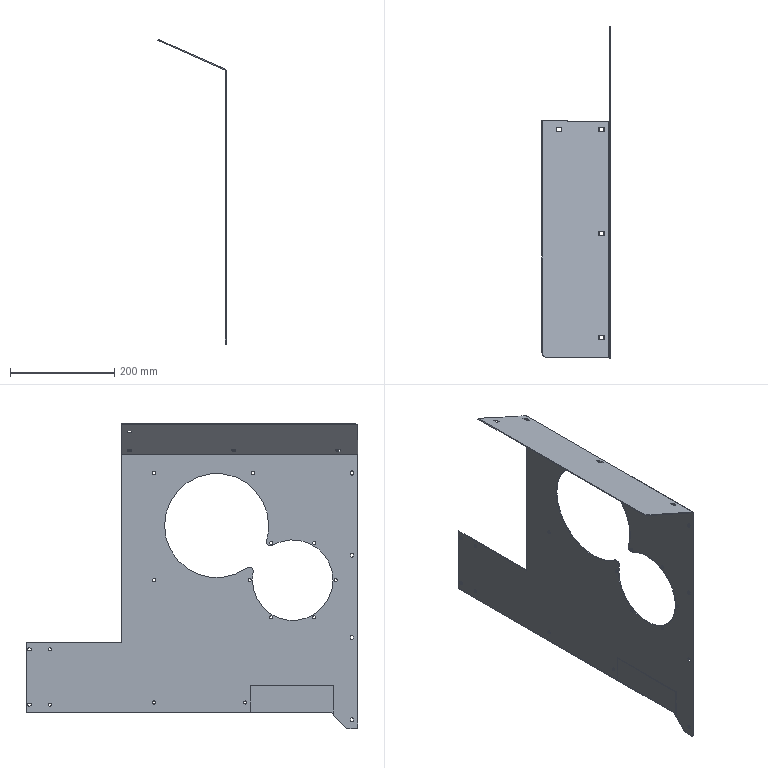Part | NX | features solid 2 | 1 solid | 119 faces | box 130.995 x 637.5 x 586.168 mm | volume 396620 mm3 | plane 62 | cylinder 57 | commonest cylinder face diameters 6 x32 5 x14 16 x3 155 x3 200 x3 3 x1